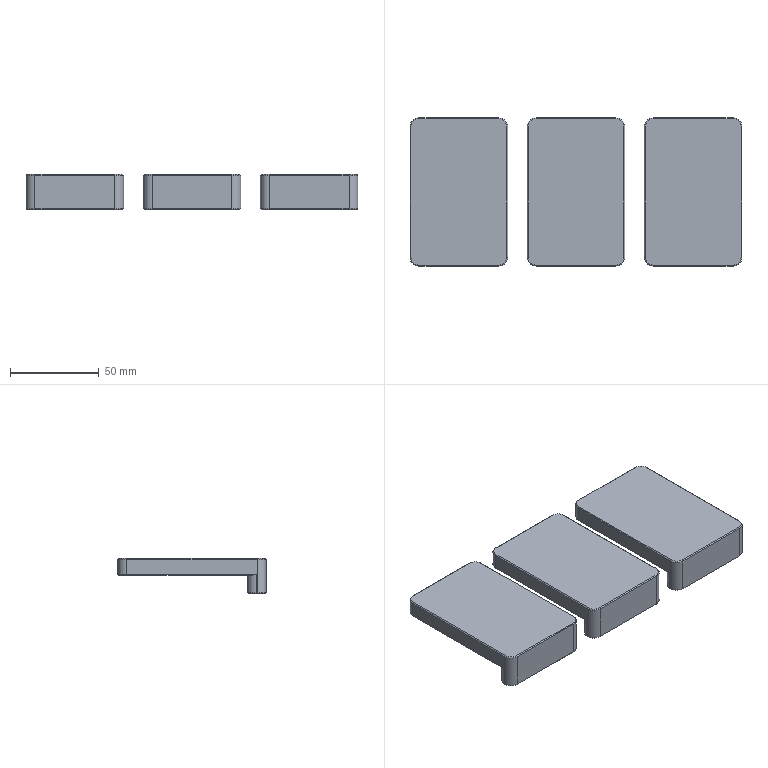Part | 3 solids | 165 faces | box 187 x 83.5 x 20 mm | volume 144134 mm3 | plane 69 | cone 54 | cylinder 42 | commonest cylinder face diameters 6 x24 10 x18